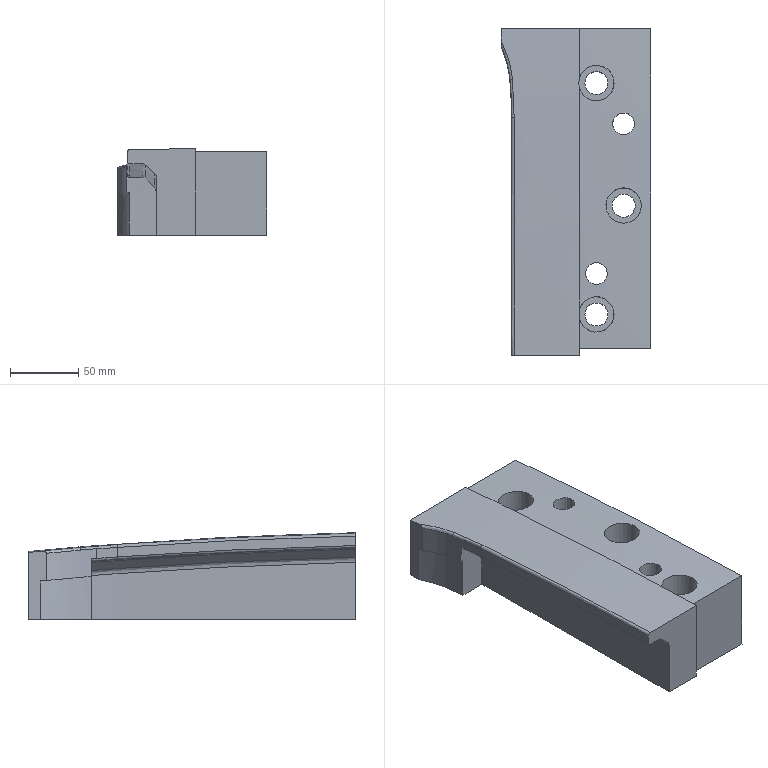Part | NX | features MAIN_BODY 2 | 1 solid | 41 faces | box 110 x 240 x 63.58 mm | volume 1103766 mm3 | spline 17 | plane 15 | cylinder 9 | commonest cylinder face diameters 17 x3 26 x3 16 x2 3.403 x1